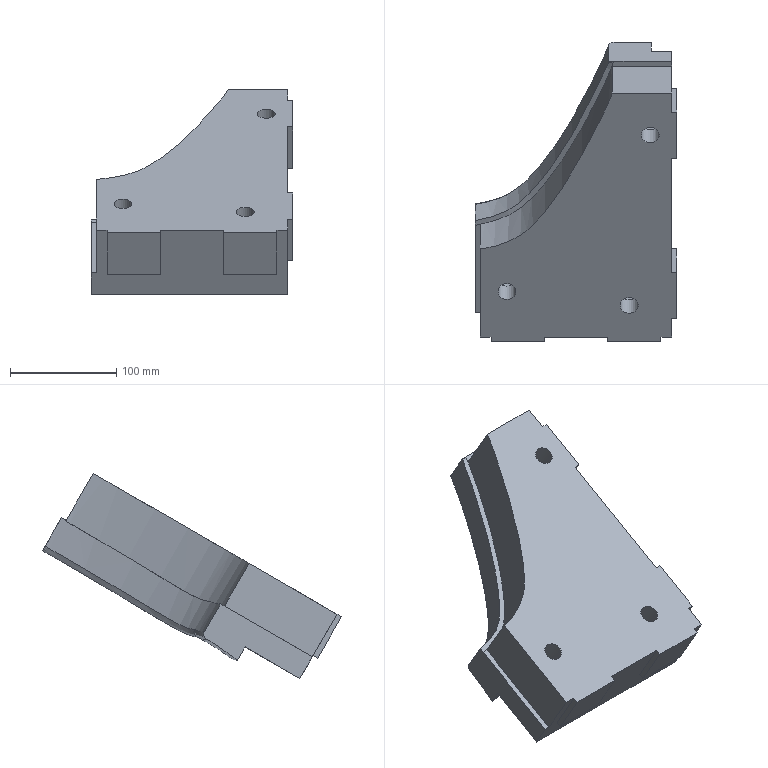Part | NX | features solid 2 | 1 solid | 44 faces | box 190 x 281.634 x 193.122 mm | volume 2521905 mm3 | plane 28 | spline 10 | cylinder 6 | commonest cylinder face diameters 17 x3 25 x3